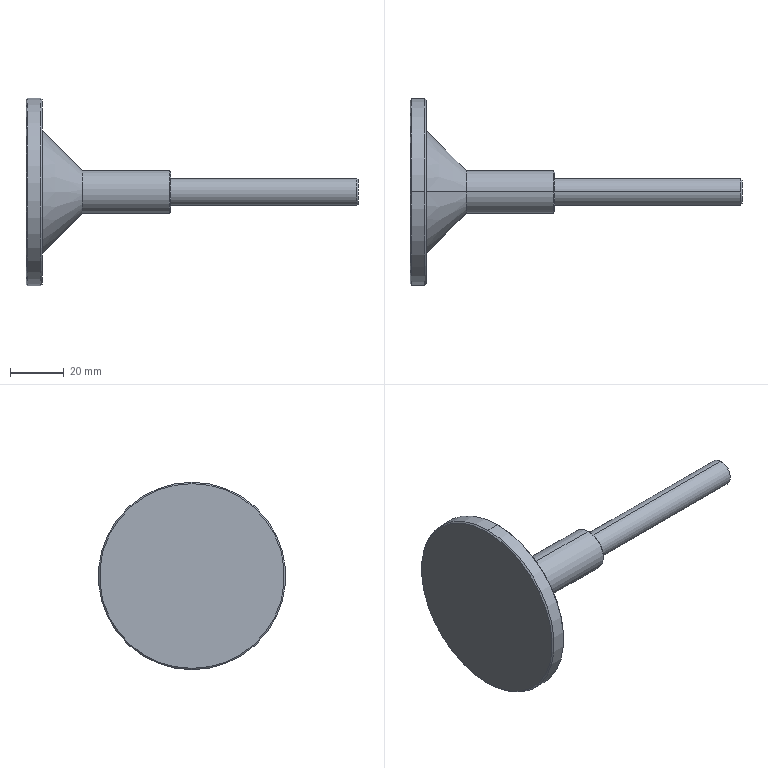Part | SolidWorks | features Chamfer 3, Revolution 1 | 1 solid | 20 faces | box 124 x 70 x 70 mm | volume 47364 mm3 | cone 10 | cylinder 6 | plane 4 | commonest cylinder face diameters 10 x2 16 x2 70 x2
STEP:
#1=CARTESIAN_POINT('',(21.,0.,-8.));
#2=VERTEX_POINT('',#1);
#3=CARTESIAN_POINT('',(21.,0.,8.));
#4=VERTEX_POINT('',#3);
#5=CARTESIAN_POINT('',(21.,0.,0.));
#6=DIRECTION('',(1.,0.,0.));
#7=DIRECTION('',(0.,0.,1.));
#8=AXIS2_PLACEMENT_3D('',#5,#6,#7);
#9=CIRCLE('',#8,8.);
#10=EDGE_CURVE('',#2,#4,#9,.T.);
#11=ORIENTED_EDGE('',*,*,#10,.F.);
#12=CARTESIAN_POINT('',(6.,0.,-23.));
#13=VERTEX_POINT('',#12);
#14=CARTESIAN_POINT('',(6.,0.,-23.));
#15=DIRECTION('',(-0.7071,0.,-0.7071));
#16=VECTOR('',#15,1000.);
#17=LINE('',#14,#16);
#18=EDGE_CURVE('',#2,#13,#17,.T.);
#19=ORIENTED_EDGE('',*,*,#18,.T.);
#20=CARTESIAN_POINT('',(6.,0.,23.));
#21=VERTEX_POINT('',#20);
#22=CARTESIAN_POINT('',(6.,0.,0.));
#23=DIRECTION('',(-1.,0.,0.));
#24=DIRECTION('',(0.,0.,1.));
#25=AXIS2_PLACEMENT_3D('',#22,#23,#24);
#26=CIRCLE('',#25,23.);
#27=EDGE_CURVE('',#21,#13,#26,.T.);
#28=ORIENTED_EDGE('',*,*,#27,.F.);
#29=CARTESIAN_POINT('',(6.,0.,23.));
#30=DIRECTION('',(-0.7071,0.,0.7071));
#31=VECTOR('',#30,1000.);
#32=LINE('',#29,#31);
#33=EDGE_CURVE('',#4,#21,#32,.T.);
#34=ORIENTED_EDGE('',*,*,#33,.F.);
#35=EDGE_LOOP('',(#11,#19,#28,#34));
#36=FACE_OUTER_BOUND('',#35,.T.);
#37=CARTESIAN_POINT('',(6.,0.,0.));
#38=DIRECTION('',(-1.,0.,0.));
#39=DIRECTION('',(0.,0.,1.));
#40=AXIS2_PLACEMENT_3D('',#37,#38,#39);
#41=CONICAL_SURFACE('',#40,23.,0.7854);
#42=ADVANCED_FACE('',(#36),#41,.T.);
#43=CARTESIAN_POINT('',(124.,0.,-4.5));
#44=VERTEX_POINT('',#43);
#45=CARTESIAN_POINT('',(124.,0.,4.5));
#46=VERTEX_POINT('',#45);
#47=CARTESIAN_POINT('',(124.,0.,0.));
#48=DIRECTION('',(1.,0.,0.));
#49=DIRECTION('',(0.,0.,1.));
#50=AXIS2_PLACEMENT_3D('',#47,#48,#49);
#51=CIRCLE('',#50,4.5);
#52=EDGE_CURVE('',#44,#46,#51,.T.);
#53=ORIENTED_EDGE('',*,*,#52,.F.);
#54=CARTESIAN_POINT('',(123.5,0.,-5.));
#55=VERTEX_POINT('',#54);
#56=CARTESIAN_POINT('',(123.5,0.,-5.));
#57=DIRECTION('',(-0.7071,0.,-0.7071));
#58=VECTOR('',#57,1000.);
#59=LINE('',#56,#58);
#60=EDGE_CURVE('',#44,#55,#59,.T.);
#61=ORIENTED_EDGE('',*,*,#60,.T.);
#62=CARTESIAN_POINT('',(123.5,0.,5.));
#63=VERTEX_POINT('',#62);
#64=CARTESIAN_POINT('',(123.5,0.,0.));
#65=DIRECTION('',(-1.,0.,0.));
#66=DIRECTION('',(0.,0.,1.));
#67=AXIS2_PLACEMENT_3D('',#64,#65,#66);
#68=CIRCLE('',#67,5.);
#69=EDGE_CURVE('',#63,#55,#68,.T.);
#70=ORIENTED_EDGE('',*,*,#69,.F.);
#71=CARTESIAN_POINT('',(123.5,0.,5.));
#72=DIRECTION('',(-0.7071,0.,0.7071));
#73=VECTOR('',#72,1000.);
#74=LINE('',#71,#73);
#75=EDGE_CURVE('',#46,#63,#74,.T.);
#76=ORIENTED_EDGE('',*,*,#75,.F.);
#77=EDGE_LOOP('',(#53,#61,#70,#76));
#78=FACE_OUTER_BOUND('',#77,.T.);
#79=CARTESIAN_POINT('',(123.5,0.,0.));
#80=DIRECTION('',(-1.,0.,0.));
#81=DIRECTION('',(0.,0.,1.));
#82=AXIS2_PLACEMENT_3D('',#79,#80,#81);
#83=CONICAL_SURFACE('',#82,5.,0.7854);
#84=ADVANCED_FACE('',(#78),#83,.T.);
#85=CARTESIAN_POINT('',(0.,0.,34.5));
#86=VERTEX_POINT('',#85);
#87=CARTESIAN_POINT('',(0.,0.,-34.5));
#88=VERTEX_POINT('',#87);
#89=CARTESIAN_POINT('',(0.,0.,0.));
#90=DIRECTION('',(-1.,0.,0.));
#91=DIRECTION('',(0.,0.,-1.));
#92=AXIS2_PLACEMENT_3D('',#89,#90,#91);
#93=CIRCLE('',#92,34.5);
#94=EDGE_CURVE('',#86,#88,#93,.T.);
#95=ORIENTED_EDGE('',*,*,#94,.F.);
#96=CARTESIAN_POINT('',(0.5,0.,35.));
#97=VERTEX_POINT('',#96);
#98=CARTESIAN_POINT('',(0.,0.,34.5));
#99=DIRECTION('',(0.7071,0.,0.7071));
#100=VECTOR('',#99,1000.);
#101=LINE('',#98,#100);
#102=EDGE_CURVE('',#86,#97,#101,.T.);
#103=ORIENTED_EDGE('',*,*,#102,.T.);
#104=CARTESIAN_POINT('',(0.5,0.,-35.));
#105=VERTEX_POINT('',#104);
#106=CARTESIAN_POINT('',(0.5,0.,0.));
#107=DIRECTION('',(1.,0.,0.));
#108=DIRECTION('',(0.,0.,-1.));
#109=AXIS2_PLACEMENT_3D('',#106,#107,#108);
#110=CIRCLE('',#109,35.);
#111=EDGE_CURVE('',#105,#97,#110,.T.);
#112=ORIENTED_EDGE('',*,*,#111,.F.);
#113=CARTESIAN_POINT('',(0.,0.,-34.5));
#114=DIRECTION('',(0.7071,0.,-0.7071));
#115=VECTOR('',#114,1000.);
#116=LINE('',#113,#115);
#117=EDGE_CURVE('',#88,#105,#116,.T.);
#118=ORIENTED_EDGE('',*,*,#117,.F.);
#119=EDGE_LOOP('',(#95,#103,#112,#118));
#120=FACE_OUTER_BOUND('',#119,.T.);
#121=CARTESIAN_POINT('',(0.,0.,0.));
#122=DIRECTION('',(1.,0.,0.));
#123=DIRECTION('',(0.,0.,-1.));
#124=AXIS2_PLACEMENT_3D('',#121,#122,#123);
#125=CONICAL_SURFACE('',#124,34.5,0.7854);
#126=ADVANCED_FACE('',(#120),#125,.T.);
#127=CARTESIAN_POINT('',(6.,0.,-34.5));
#128=VERTEX_POINT('',#127);
#129=CARTESIAN_POINT('',(6.,0.,34.5));
#130=VERTEX_POINT('',#129);
#131=CARTESIAN_POINT('',(6.,0.,0.));
#132=DIRECTION('',(1.,0.,0.));
#133=DIRECTION('',(0.,0.,1.));
#134=AXIS2_PLACEMENT_3D('',#131,#132,#133);
#135=CIRCLE('',#134,34.5);
#136=EDGE_CURVE('',#128,#130,#135,.T.);
#137=ORIENTED_EDGE('',*,*,#136,.F.);
#138=CARTESIAN_POINT('',(5.5,0.,-35.));
#139=VERTEX_POINT('',#138);
#140=CARTESIAN_POINT('',(5.5,0.,-35.));
#141=DIRECTION('',(-0.7071,0.,-0.7071));
#142=VECTOR('',#141,1000.);
#143=LINE('',#140,#142);
#144=EDGE_CURVE('',#128,#139,#143,.T.);
#145=ORIENTED_EDGE('',*,*,#144,.T.);
#146=CARTESIAN_POINT('',(5.5,0.,35.));
#147=VERTEX_POINT('',#146);
#148=CARTESIAN_POINT('',(5.5,0.,0.));
#149=DIRECTION('',(-1.,0.,0.));
#150=DIRECTION('',(0.,0.,1.));
#151=AXIS2_PLACEMENT_3D('',#148,#149,#150);
#152=CIRCLE('',#151,35.);
#153=EDGE_CURVE('',#147,#139,#152,.T.);
#154=ORIENTED_EDGE('',*,*,#153,.F.);
#155=CARTESIAN_POINT('',(5.5,0.,35.));
#156=DIRECTION('',(-0.7071,0.,0.7071));
#157=VECTOR('',#156,1000.);
#158=LINE('',#155,#157);
#159=EDGE_CURVE('',#130,#147,#158,.T.);
#160=ORIENTED_EDGE('',*,*,#159,.F.);
#161=EDGE_LOOP('',(#137,#145,#154,#160));
#162=FACE_OUTER_BOUND('',#161,.T.);
#163=CARTESIAN_POINT('',(5.5,0.,0.));
#164=DIRECTION('',(-1.,0.,0.));
#165=DIRECTION('',(0.,0.,1.));
#166=AXIS2_PLACEMENT_3D('',#163,#164,#165);
#167=CONICAL_SURFACE('',#166,35.,0.7854);
#168=ADVANCED_FACE('',(#162),#167,.T.);
#169=CARTESIAN_POINT('',(54.,0.,-7.5));
#170=VERTEX_POINT('',#169);
#171=CARTESIAN_POINT('',(54.,0.,7.5));
#172=VERTEX_POINT('',#171);
#173=CARTESIAN_POINT('',(54.,0.,0.));
#174=DIRECTION('',(1.,0.,0.));
#175=DIRECTION('',(0.,0.,1.));
#176=AXIS2_PLACEMENT_3D('',#173,#174,#175);
#177=CIRCLE('',#176,7.5);
#178=EDGE_CURVE('',#170,#172,#177,.T.);
#179=ORIENTED_EDGE('',*,*,#178,.F.);
#180=CARTESIAN_POINT('',(53.5,0.,-8.));
#181=VERTEX_POINT('',#180);
#182=CARTESIAN_POINT('',(53.5,0.,-8.));
#183=DIRECTION('',(-0.7071,0.,-0.7071));
#184=VECTOR('',#183,1000.);
#185=LINE('',#182,#184);
#186=EDGE_CURVE('',#170,#181,#185,.T.);
#187=ORIENTED_EDGE('',*,*,#186,.T.);
#188=CARTESIAN_POINT('',(53.5,0.,8.));
#189=VERTEX_POINT('',#188);
#190=CARTESIAN_POINT('',(53.5,0.,0.));
#191=DIRECTION('',(-1.,0.,0.));
#192=DIRECTION('',(0.,0.,1.));
#193=AXIS2_PLACEMENT_3D('',#190,#191,#192);
#194=CIRCLE('',#193,8.);
#195=EDGE_CURVE('',#189,#181,#194,.T.);
#196=ORIENTED_EDGE('',*,*,#195,.F.);
#197=CARTESIAN_POINT('',(53.5,0.,8.));
#198=DIRECTION('',(-0.7071,0.,0.7071));
#199=VECTOR('',#198,1000.);
#200=LINE('',#197,#199);
#201=EDGE_CURVE('',#172,#189,#200,.T.);
#202=ORIENTED_EDGE('',*,*,#201,.F.);
#203=EDGE_LOOP('',(#179,#187,#196,#202));
#204=FACE_OUTER_BOUND('',#203,.T.);
#205=CARTESIAN_POINT('',(53.5,0.,0.));
#206=DIRECTION('',(-1.,0.,0.));
#207=DIRECTION('',(0.,0.,1.));
#208=AXIS2_PLACEMENT_3D('',#205,#206,#207);
#209=CONICAL_SURFACE('',#208,8.,0.7854);
#210=ADVANCED_FACE('',(#204),#209,.T.);
#211=ORIENTED_EDGE('',*,*,#69,.T.);
#212=CARTESIAN_POINT('',(54.,0.,-5.));
#213=VERTEX_POINT('',#212);
#214=CARTESIAN_POINT('',(0.,0.,-5.));
#215=DIRECTION('',(-1.,0.,0.));
#216=VECTOR('',#215,1000.);
#217=LINE('',#214,#216);
#218=EDGE_CURVE('',#55,#213,#217,.T.);
#219=ORIENTED_EDGE('',*,*,#218,.T.);
#220=CARTESIAN_POINT('',(54.,0.,5.));
#221=VERTEX_POINT('',#220);
#222=CARTESIAN_POINT('',(54.,0.,0.));
#223=DIRECTION('',(-1.,0.,0.));
#224=DIRECTION('',(0.,0.,1.));
#225=AXIS2_PLACEMENT_3D('',#222,#223,#224);
#226=CIRCLE('',#225,5.);
#227=EDGE_CURVE('',#221,#213,#226,.T.);
#228=ORIENTED_EDGE('',*,*,#227,.F.);
#229=CARTESIAN_POINT('',(0.,0.,5.));
#230=DIRECTION('',(-1.,0.,0.));
#231=VECTOR('',#230,1000.);
#232=LINE('',#229,#231);
#233=EDGE_CURVE('',#63,#221,#232,.T.);
#234=ORIENTED_EDGE('',*,*,#233,.F.);
#235=EDGE_LOOP('',(#211,#219,#228,#234));
#236=FACE_OUTER_BOUND('',#235,.T.);
#237=CARTESIAN_POINT('',(0.,0.,0.));
#238=DIRECTION('',(-1.,0.,0.));
#239=DIRECTION('',(0.,0.,1.));
#240=AXIS2_PLACEMENT_3D('',#237,#238,#239);
#241=CYLINDRICAL_SURFACE('',#240,5.);
#242=ADVANCED_FACE('',(#236),#241,.T.);
#243=ORIENTED_EDGE('',*,*,#195,.T.);
#244=CARTESIAN_POINT('',(0.,0.,-8.));
#245=DIRECTION('',(-1.,0.,0.));
#246=VECTOR('',#245,1000.);
#247=LINE('',#244,#246);
#248=EDGE_CURVE('',#181,#2,#247,.T.);
#249=ORIENTED_EDGE('',*,*,#248,.T.);
#250=ORIENTED_EDGE('',*,*,#10,.T.);
#251=CARTESIAN_POINT('',(0.,0.,8.));
#252=DIRECTION('',(-1.,0.,0.));
#253=VECTOR('',#252,1000.);
#254=LINE('',#251,#253);
#255=EDGE_CURVE('',#189,#4,#254,.T.);
#256=ORIENTED_EDGE('',*,*,#255,.F.);
#257=EDGE_LOOP('',(#243,#249,#250,#256));
#258=FACE_OUTER_BOUND('',#257,.T.);
#259=CARTESIAN_POINT('',(0.,0.,0.));
#260=DIRECTION('',(-1.,0.,0.));
#261=DIRECTION('',(0.,0.,1.));
#262=AXIS2_PLACEMENT_3D('',#259,#260,#261);
#263=CYLINDRICAL_SURFACE('',#262,8.);
#264=ADVANCED_FACE('',(#258),#263,.T.);
#265=ORIENTED_EDGE('',*,*,#153,.T.);
#266=CARTESIAN_POINT('',(0.,0.,-35.));
#267=DIRECTION('',(-1.,0.,0.));
#268=VECTOR('',#267,1000.);
#269=LINE('',#266,#268);
#270=EDGE_CURVE('',#139,#105,#269,.T.);
#271=ORIENTED_EDGE('',*,*,#270,.T.);
#272=ORIENTED_EDGE('',*,*,#111,.T.);
#273=CARTESIAN_POINT('',(0.,0.,35.));
#274=DIRECTION('',(-1.,0.,0.));
#275=VECTOR('',#274,1000.);
#276=LINE('',#273,#275);
#277=EDGE_CURVE('',#147,#97,#276,.T.);
#278=ORIENTED_EDGE('',*,*,#277,.F.);
#279=EDGE_LOOP('',(#265,#271,#272,#278));
#280=FACE_OUTER_BOUND('',#279,.T.);
#281=CARTESIAN_POINT('',(0.,0.,0.));
#282=DIRECTION('',(-1.,0.,0.));
#283=DIRECTION('',(0.,0.,1.));
#284=AXIS2_PLACEMENT_3D('',#281,#282,#283);
#285=CYLINDRICAL_SURFACE('',#284,35.);
#286=ADVANCED_FACE('',(#280),#285,.T.);
#287=CARTESIAN_POINT('',(0.,0.,0.));
#288=DIRECTION('',(-1.,0.,0.));
#289=DIRECTION('',(0.,0.,-1.));
#290=AXIS2_PLACEMENT_3D('',#287,#288,#289);
#291=CIRCLE('',#290,34.5);
#292=EDGE_CURVE('',#88,#86,#291,.T.);
#293=ORIENTED_EDGE('',*,*,#292,.T.);
#294=ORIENTED_EDGE('',*,*,#94,.T.);
#295=EDGE_LOOP('',(#293,#294));
#296=FACE_OUTER_BOUND('',#295,.T.);
#297=CARTESIAN_POINT('',(0.,0.,0.));
#298=DIRECTION('',(1.,0.,0.));
#299=DIRECTION('',(0.,0.,-1.));
#300=AXIS2_PLACEMENT_3D('',#297,#298,#299);
#301=PLANE('',#300);
#302=ADVANCED_FACE('',(#296),#301,.F.);
#303=ORIENTED_EDGE('',*,*,#270,.F.);
#304=CARTESIAN_POINT('',(5.5,0.,0.));
#305=DIRECTION('',(-1.,0.,0.));
#306=DIRECTION('',(0.,0.,1.));
#307=AXIS2_PLACEMENT_3D('',#304,#305,#306);
#308=CIRCLE('',#307,35.);
#309=EDGE_CURVE('',#139,#147,#308,.T.);
#310=ORIENTED_EDGE('',*,*,#309,.T.);
#311=ORIENTED_EDGE('',*,*,#277,.T.);
#312=CARTESIAN_POINT('',(0.5,0.,0.));
#313=DIRECTION('',(1.,0.,0.));
#314=DIRECTION('',(0.,0.,-1.));
#315=AXIS2_PLACEMENT_3D('',#312,#313,#314);
#316=CIRCLE('',#315,35.);
#317=EDGE_CURVE('',#97,#105,#316,.T.);
#318=ORIENTED_EDGE('',*,*,#317,.T.);
#319=EDGE_LOOP('',(#303,#310,#311,#318));
#320=FACE_OUTER_BOUND('',#319,.T.);
#321=CARTESIAN_POINT('',(0.,0.,0.));
#322=DIRECTION('',(-1.,0.,0.));
#323=DIRECTION('',(0.,0.,1.));
#324=AXIS2_PLACEMENT_3D('',#321,#322,#323);
#325=CYLINDRICAL_SURFACE('',#324,35.);
#326=ADVANCED_FACE('',(#320),#325,.T.);
#327=ORIENTED_EDGE('',*,*,#27,.T.);
#328=CARTESIAN_POINT('',(6.,0.,0.));
#329=DIRECTION('',(-1.,0.,0.));
#330=DIRECTION('',(0.,0.,1.));
#331=AXIS2_PLACEMENT_3D('',#328,#329,#330);
#332=CIRCLE('',#331,23.);
#333=EDGE_CURVE('',#13,#21,#332,.T.);
#334=ORIENTED_EDGE('',*,*,#333,.T.);
#335=EDGE_LOOP('',(#327,#334));
#336=FACE_BOUND('',#335,.T.);
#337=CARTESIAN_POINT('',(6.,0.,0.));
#338=DIRECTION('',(1.,0.,0.));
#339=DIRECTION('',(0.,0.,1.));
#340=AXIS2_PLACEMENT_3D('',#337,#338,#339);
#341=CIRCLE('',#340,34.5);
#342=EDGE_CURVE('',#130,#128,#341,.T.);
#343=ORIENTED_EDGE('',*,*,#342,.T.);
#344=ORIENTED_EDGE('',*,*,#136,.T.);
#345=EDGE_LOOP('',(#343,#344));
#346=FACE_OUTER_BOUND('',#345,.T.);
#347=CARTESIAN_POINT('',(6.,35.,0.));
#348=DIRECTION('',(-1.,0.,0.));
#349=DIRECTION('',(0.,0.,1.));
#350=AXIS2_PLACEMENT_3D('',#347,#348,#349);
#351=PLANE('',#350);
#352=ADVANCED_FACE('',(#336,#346),#351,.F.);
#353=ORIENTED_EDGE('',*,*,#248,.F.);
#354=CARTESIAN_POINT('',(53.5,0.,0.));
#355=DIRECTION('',(-1.,0.,0.));
#356=DIRECTION('',(0.,0.,1.));
#357=AXIS2_PLACEMENT_3D('',#354,#355,#356);
#358=CIRCLE('',#357,8.);
#359=EDGE_CURVE('',#181,#189,#358,.T.);
#360=ORIENTED_EDGE('',*,*,#359,.T.);
#361=ORIENTED_EDGE('',*,*,#255,.T.);
#362=CARTESIAN_POINT('',(21.,0.,0.));
#363=DIRECTION('',(1.,0.,0.));
#364=DIRECTION('',(0.,0.,1.));
#365=AXIS2_PLACEMENT_3D('',#362,#363,#364);
#366=CIRCLE('',#365,8.);
#367=EDGE_CURVE('',#4,#2,#366,.T.);
#368=ORIENTED_EDGE('',*,*,#367,.T.);
#369=EDGE_LOOP('',(#353,#360,#361,#368));
#370=FACE_OUTER_BOUND('',#369,.T.);
#371=CARTESIAN_POINT('',(0.,0.,0.));
#372=DIRECTION('',(-1.,0.,0.));
#373=DIRECTION('',(0.,0.,1.));
#374=AXIS2_PLACEMENT_3D('',#371,#372,#373);
#375=CYLINDRICAL_SURFACE('',#374,8.);
#376=ADVANCED_FACE('',(#370),#375,.T.);
#377=CARTESIAN_POINT('',(54.,0.,0.));
#378=DIRECTION('',(1.,0.,0.));
#379=DIRECTION('',(0.,0.,1.));
#380=AXIS2_PLACEMENT_3D('',#377,#378,#379);
#381=CIRCLE('',#380,7.5);
#382=EDGE_CURVE('',#172,#170,#381,.T.);
#383=ORIENTED_EDGE('',*,*,#382,.T.);
#384=ORIENTED_EDGE('',*,*,#178,.T.);
#385=EDGE_LOOP('',(#383,#384));
#386=FACE_OUTER_BOUND('',#385,.T.);
#387=ORIENTED_EDGE('',*,*,#227,.T.);
#388=CARTESIAN_POINT('',(54.,0.,0.));
#389=DIRECTION('',(-1.,0.,0.));
#390=DIRECTION('',(0.,0.,1.));
#391=AXIS2_PLACEMENT_3D('',#388,#389,#390);
#392=CIRCLE('',#391,5.);
#393=EDGE_CURVE('',#213,#221,#392,.T.);
#394=ORIENTED_EDGE('',*,*,#393,.T.);
#395=EDGE_LOOP('',(#387,#394));
#396=FACE_BOUND('',#395,.T.);
#397=CARTESIAN_POINT('',(54.,8.,0.));
#398=DIRECTION('',(-1.,0.,0.));
#399=DIRECTION('',(0.,0.,1.));
#400=AXIS2_PLACEMENT_3D('',#397,#398,#399);
#401=PLANE('',#400);
#402=ADVANCED_FACE('',(#386,#396),#401,.F.);
#403=ORIENTED_EDGE('',*,*,#218,.F.);
#404=CARTESIAN_POINT('',(123.5,0.,0.));
#405=DIRECTION('',(-1.,0.,0.));
#406=DIRECTION('',(0.,0.,1.));
#407=AXIS2_PLACEMENT_3D('',#404,#405,#406);
#408=CIRCLE('',#407,5.);
#409=EDGE_CURVE('',#55,#63,#408,.T.);
#410=ORIENTED_EDGE('',*,*,#409,.T.);
#411=ORIENTED_EDGE('',*,*,#233,.T.);
#412=ORIENTED_EDGE('',*,*,#393,.F.);
#413=EDGE_LOOP('',(#403,#410,#411,#412));
#414=FACE_OUTER_BOUND('',#413,.T.);
#415=CARTESIAN_POINT('',(0.,0.,0.));
#416=DIRECTION('',(-1.,0.,0.));
#417=DIRECTION('',(0.,0.,1.));
#418=AXIS2_PLACEMENT_3D('',#415,#416,#417);
#419=CYLINDRICAL_SURFACE('',#418,5.);
#420=ADVANCED_FACE('',(#414),#419,.T.);
#421=CARTESIAN_POINT('',(124.,0.,0.));
#422=DIRECTION('',(1.,0.,0.));
#423=DIRECTION('',(0.,0.,1.));
#424=AXIS2_PLACEMENT_3D('',#421,#422,#423);
#425=CIRCLE('',#424,4.5);
#426=EDGE_CURVE('',#46,#44,#425,.T.);
#427=ORIENTED_EDGE('',*,*,#426,.T.);
#428=ORIENTED_EDGE('',*,*,#52,.T.);
#429=EDGE_LOOP('',(#427,#428));
#430=FACE_OUTER_BOUND('',#429,.T.);
#431=CARTESIAN_POINT('',(124.,5.,0.));
#432=DIRECTION('',(-1.,0.,0.));
#433=DIRECTION('',(0.,0.,1.));
#434=AXIS2_PLACEMENT_3D('',#431,#432,#433);
#435=PLANE('',#434);
#436=ADVANCED_FACE('',(#430),#435,.F.);
#437=ORIENTED_EDGE('',*,*,#186,.F.);
#438=ORIENTED_EDGE('',*,*,#382,.F.);
#439=ORIENTED_EDGE('',*,*,#201,.T.);
#440=ORIENTED_EDGE('',*,*,#359,.F.);
#441=EDGE_LOOP('',(#437,#438,#439,#440));
#442=FACE_OUTER_BOUND('',#441,.T.);
#443=CARTESIAN_POINT('',(53.5,0.,0.));
#444=DIRECTION('',(-1.,0.,0.));
#445=DIRECTION('',(0.,0.,1.));
#446=AXIS2_PLACEMENT_3D('',#443,#444,#445);
#447=CONICAL_SURFACE('',#446,8.,0.7854);
#448=ADVANCED_FACE('',(#442),#447,.T.);
#449=ORIENTED_EDGE('',*,*,#144,.F.);
#450=ORIENTED_EDGE('',*,*,#342,.F.);
#451=ORIENTED_EDGE('',*,*,#159,.T.);
#452=ORIENTED_EDGE('',*,*,#309,.F.);
#453=EDGE_LOOP('',(#449,#450,#451,#452));
#454=FACE_OUTER_BOUND('',#453,.T.);
#455=CARTESIAN_POINT('',(5.5,0.,0.));
#456=DIRECTION('',(-1.,0.,0.));
#457=DIRECTION('',(0.,0.,1.));
#458=AXIS2_PLACEMENT_3D('',#455,#456,#457);
#459=CONICAL_SURFACE('',#458,35.,0.7854);
#460=ADVANCED_FACE('',(#454),#459,.T.);
#461=ORIENTED_EDGE('',*,*,#102,.F.);
#462=ORIENTED_EDGE('',*,*,#292,.F.);
#463=ORIENTED_EDGE('',*,*,#117,.T.);
#464=ORIENTED_EDGE('',*,*,#317,.F.);
#465=EDGE_LOOP('',(#461,#462,#463,#464));
#466=FACE_OUTER_BOUND('',#465,.T.);
#467=CARTESIAN_POINT('',(0.,0.,0.));
#468=DIRECTION('',(1.,0.,0.));
#469=DIRECTION('',(0.,0.,-1.));
#470=AXIS2_PLACEMENT_3D('',#467,#468,#469);
#471=CONICAL_SURFACE('',#470,34.5,0.7854);
#472=ADVANCED_FACE('',(#466),#471,.T.);
#473=ORIENTED_EDGE('',*,*,#60,.F.);
#474=ORIENTED_EDGE('',*,*,#426,.F.);
#475=ORIENTED_EDGE('',*,*,#75,.T.);
#476=ORIENTED_EDGE('',*,*,#409,.F.);
#477=EDGE_LOOP('',(#473,#474,#475,#476));
#478=FACE_OUTER_BOUND('',#477,.T.);
#479=CARTESIAN_POINT('',(123.5,0.,0.));
#480=DIRECTION('',(-1.,0.,0.));
#481=DIRECTION('',(0.,0.,1.));
#482=AXIS2_PLACEMENT_3D('',#479,#480,#481);
#483=CONICAL_SURFACE('',#482,5.,0.7854);
#484=ADVANCED_FACE('',(#478),#483,.T.);
#485=ORIENTED_EDGE('',*,*,#18,.F.);
#486=ORIENTED_EDGE('',*,*,#367,.F.);
#487=ORIENTED_EDGE('',*,*,#33,.T.);
#488=ORIENTED_EDGE('',*,*,#333,.F.);
#489=EDGE_LOOP('',(#485,#486,#487,#488));
#490=FACE_OUTER_BOUND('',#489,.T.);
#491=CARTESIAN_POINT('',(6.,0.,0.));
#492=DIRECTION('',(-1.,0.,0.));
#493=DIRECTION('',(0.,0.,1.));
#494=AXIS2_PLACEMENT_3D('',#491,#492,#493);
#495=CONICAL_SURFACE('',#494,23.,0.7854);
#496=ADVANCED_FACE('',(#490),#495,.T.);
#497=CLOSED_SHELL('',(#42,#84,#126,#168,#210,#242,#264,#286,#302,#326,#352,#376,#402,#420,#436,#448,#460,#472,#484,#496));
#498=MANIFOLD_SOLID_BREP('',#497);
#499=CARTESIAN_POINT('',(0.,0.,0.));
#500=DIRECTION('',(0.,0.,1.));
#501=DIRECTION('',(1.,0.,0.));
#502=AXIS2_PLACEMENT_3D('',#499,#500,#501);
#503=(LENGTH_UNIT()NAMED_UNIT(*)SI_UNIT(.MILLI.,.METRE.));
#504=UNCERTAINTY_MEASURE_WITH_UNIT(LENGTH_MEASURE(0.00001),#503,'','');
#505=(NAMED_UNIT(*)PLANE_ANGLE_UNIT()SI_UNIT($,.RADIAN.));
#506=(NAMED_UNIT(*)SI_UNIT($,.STERADIAN.)SOLID_ANGLE_UNIT());
#507=(GEOMETRIC_REPRESENTATION_CONTEXT(3)GLOBAL_UNCERTAINTY_ASSIGNED_CONTEXT((#504))GLOBAL_UNIT_ASSIGNED_CONTEXT((#503,#505,#506))REPRESENTATION_CONTEXT('',''));
#508=ADVANCED_BREP_SHAPE_REPRESENTATION('',(#498,#502),#507);